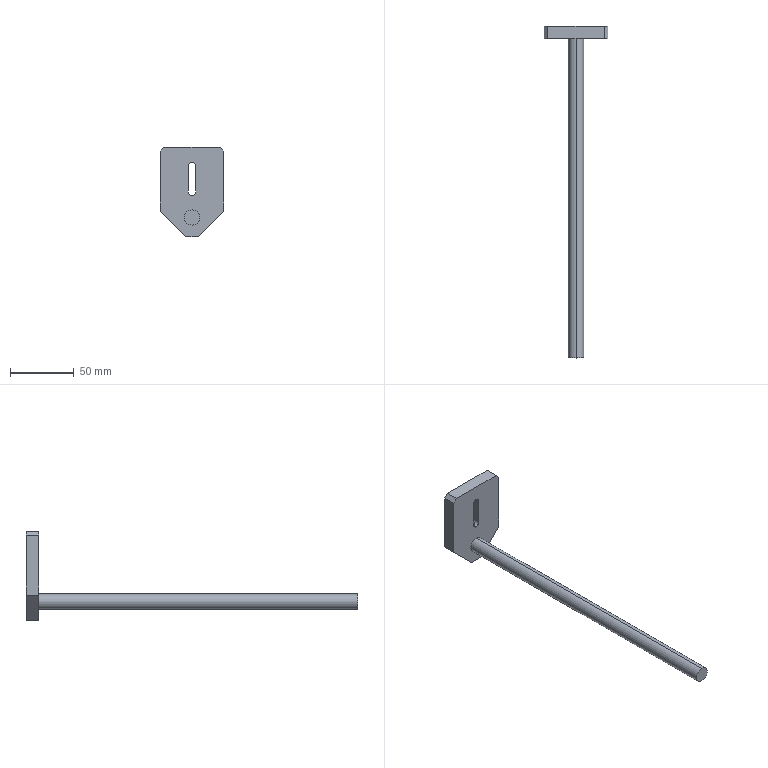Part | SolidWorks | features ICE 3, Chamfer 1, Extrusion 1, HoleWzd 1 | 1 solid | 20 faces | box 50 x 260 x 70 mm | volume 57256 mm3 | plane 13 | cylinder 7 | commonest cylinder face diameters 6 x3 4.2 x2 12 x2
STEP:
#1=CARTESIAN_POINT('',(2.1,5.,-12.142));
#2=VERTEX_POINT('',#1);
#3=CARTESIAN_POINT('',(0.,2.9,-13.));
#4=VERTEX_POINT('',#3);
#5=CARTESIAN_POINT('',(2.1,5.,-12.142));
#6=CARTESIAN_POINT('',(2.1,4.858,-12.142));
#7=CARTESIAN_POINT('',(2.085,4.714,-12.157));
#8=CARTESIAN_POINT('',(2.028,4.438,-12.211));
#9=CARTESIAN_POINT('',(1.986,4.305,-12.249));
#10=CARTESIAN_POINT('',(1.88,4.054,-12.339));
#11=CARTESIAN_POINT('',(1.816,3.937,-12.39));
#12=CARTESIAN_POINT('',(1.668,3.718,-12.495));
#13=CARTESIAN_POINT('',(1.583,3.614,-12.551));
#14=CARTESIAN_POINT('',(1.396,3.426,-12.657));
#15=CARTESIAN_POINT('',(1.295,3.341,-12.709));
#16=CARTESIAN_POINT('',(1.072,3.189,-12.804));
#17=CARTESIAN_POINT('',(0.9508,3.123,-12.848));
#18=CARTESIAN_POINT('',(0.6972,3.014,-12.921));
#19=CARTESIAN_POINT('',(0.5628,2.972,-12.95));
#20=CARTESIAN_POINT('',(0.2837,2.914,-12.99));
#21=CARTESIAN_POINT('',(0.1426,2.9,-13.));
#22=CARTESIAN_POINT('',(0.,2.9,-13.));
#23=B_SPLINE_CURVE_WITH_KNOTS('',3,(#5,#6,#7,#8,#9,#10,#11,#12,#13,#14,#15,#16,#17,#18,#19,#20,#21,#22),.UNSPECIFIED.,.F.,.F.,(4,2,2,2,2,2,2,2,4),(0.006811,0.007236,0.007662,0.008087,0.008512,0.008938,0.009363,0.009789,0.01021),.UNSPECIFIED.);
#24=EDGE_CURVE('',#2,#4,#23,.T.);
#25=ORIENTED_EDGE('',*,*,#24,.F.);
#26=CARTESIAN_POINT('',(2.1,5.,-45.));
#27=VERTEX_POINT('',#26);
#28=CARTESIAN_POINT('',(2.1,5.,-45.));
#29=DIRECTION('',(0.,0.,-1.));
#30=VECTOR('',#29,1000.);
#31=LINE('',#28,#30);
#32=EDGE_CURVE('',#2,#27,#31,.T.);
#33=ORIENTED_EDGE('',*,*,#32,.T.);
#34=CARTESIAN_POINT('',(-2.1,5.,-45.));
#35=VERTEX_POINT('',#34);
#36=CARTESIAN_POINT('',(0.,5.,-45.));
#37=DIRECTION('',(0.,0.,-1.));
#38=DIRECTION('',(-1.,0.,0.));
#39=AXIS2_PLACEMENT_3D('',#36,#37,#38);
#40=CIRCLE('',#39,2.1);
#41=EDGE_CURVE('',#27,#35,#40,.T.);
#42=ORIENTED_EDGE('',*,*,#41,.T.);
#43=CARTESIAN_POINT('',(-2.1,5.,-12.142));
#44=VERTEX_POINT('',#43);
#45=CARTESIAN_POINT('',(-2.1,5.,-45.));
#46=DIRECTION('',(0.,0.,-1.));
#47=VECTOR('',#46,1000.);
#48=LINE('',#45,#47);
#49=EDGE_CURVE('',#44,#35,#48,.T.);
#50=ORIENTED_EDGE('',*,*,#49,.F.);
#51=CARTESIAN_POINT('',(0.,2.9,-13.));
#52=CARTESIAN_POINT('',(-0.1424,2.9,-13.));
#53=CARTESIAN_POINT('',(-0.2871,2.915,-12.989));
#54=CARTESIAN_POINT('',(-0.5634,2.972,-12.95));
#55=CARTESIAN_POINT('',(-0.6985,3.015,-12.921));
#56=CARTESIAN_POINT('',(-1.081,3.178,-12.811));
#57=CARTESIAN_POINT('',(-1.306,3.334,-12.709));
#58=CARTESIAN_POINT('',(-1.678,3.71,-12.496));
#59=CARTESIAN_POINT('',(-1.828,3.933,-12.382));
#60=CARTESIAN_POINT('',(-1.986,4.305,-12.249));
#61=CARTESIAN_POINT('',(-2.028,4.438,-12.211));
#62=CARTESIAN_POINT('',(-2.085,4.714,-12.157));
#63=CARTESIAN_POINT('',(-2.1,4.856,-12.142));
#64=CARTESIAN_POINT('',(-2.1,5.,-12.142));
#65=B_SPLINE_CURVE_WITH_KNOTS('',3,(#51,#52,#53,#54,#55,#56,#57,#58,#59,#60,#61,#62,#63,#64),.UNSPECIFIED.,.F.,.F.,(4,2,2,2,2,2,4),(0.01021,0.01064,0.01106,0.01191,0.01276,0.01319,0.01361),.UNSPECIFIED.);
#66=EDGE_CURVE('',#4,#44,#65,.T.);
#67=ORIENTED_EDGE('',*,*,#66,.F.);
#68=EDGE_LOOP('',(#25,#33,#42,#50,#67));
#69=FACE_OUTER_BOUND('',#68,.T.);
#70=CARTESIAN_POINT('',(0.,5.,-45.));
#71=DIRECTION('',(0.,0.,-1.));
#72=DIRECTION('',(-1.,0.,0.));
#73=AXIS2_PLACEMENT_3D('',#70,#71,#72);
#74=CYLINDRICAL_SURFACE('',#73,2.1);
#75=ADVANCED_FACE('',(#69),#74,.F.);
#76=CARTESIAN_POINT('',(0.,10.,-13.));
#77=VERTEX_POINT('',#76);
#78=CARTESIAN_POINT('',(3.,10.,-10.));
#79=VERTEX_POINT('',#78);
#80=CARTESIAN_POINT('',(0.,10.,-10.));
#81=DIRECTION('',(0.,-1.,0.));
#82=DIRECTION('',(0.,0.,-1.));
#83=AXIS2_PLACEMENT_3D('',#80,#81,#82);
#84=CIRCLE('',#83,3.);
#85=EDGE_CURVE('',#77,#79,#84,.T.);
#86=ORIENTED_EDGE('',*,*,#85,.F.);
#87=CARTESIAN_POINT('',(0.,7.1,-13.));
#88=VERTEX_POINT('',#87);
#89=CARTESIAN_POINT('',(0.,10.,-13.));
#90=DIRECTION('',(0.,-1.,0.));
#91=VECTOR('',#90,1000.);
#92=LINE('',#89,#91);
#93=EDGE_CURVE('',#77,#88,#92,.T.);
#94=ORIENTED_EDGE('',*,*,#93,.T.);
#95=CARTESIAN_POINT('',(0.,7.1,-13.));
#96=CARTESIAN_POINT('',(0.1432,7.1,-13.));
#97=CARTESIAN_POINT('',(0.2844,7.086,-12.99));
#98=CARTESIAN_POINT('',(0.5628,7.028,-12.95));
#99=CARTESIAN_POINT('',(0.6977,6.986,-12.921));
#100=CARTESIAN_POINT('',(0.9516,6.877,-12.848));
#101=CARTESIAN_POINT('',(1.073,6.81,-12.804));
#102=CARTESIAN_POINT('',(1.295,6.658,-12.709));
#103=CARTESIAN_POINT('',(1.397,6.573,-12.657));
#104=CARTESIAN_POINT('',(1.679,6.289,-12.495));
#105=CARTESIAN_POINT('',(1.828,6.07,-12.383));
#106=CARTESIAN_POINT('',(1.987,5.692,-12.249));
#107=CARTESIAN_POINT('',(2.028,5.561,-12.211));
#108=CARTESIAN_POINT('',(2.085,5.285,-12.157));
#109=CARTESIAN_POINT('',(2.1,5.142,-12.142));
#110=CARTESIAN_POINT('',(2.1,5.,-12.142));
#111=B_SPLINE_CURVE_WITH_KNOTS('',3,(#95,#96,#97,#98,#99,#100,#101,#102,#103,#104,#105,#106,#107,#108,#109,#110),.UNSPECIFIED.,.F.,.F.,(4,2,2,2,2,2,2,4),(0.003408,0.003833,0.004259,0.004684,0.005109,0.00596,0.006386,0.006811),.UNSPECIFIED.);
#112=EDGE_CURVE('',#88,#2,#111,.T.);
#113=ORIENTED_EDGE('',*,*,#112,.T.);
#114=ORIENTED_EDGE('',*,*,#24,.T.);
#115=CARTESIAN_POINT('',(0.,0.,-13.));
#116=VERTEX_POINT('',#115);
#117=CARTESIAN_POINT('',(0.,10.,-13.));
#118=DIRECTION('',(0.,-1.,0.));
#119=VECTOR('',#118,1000.);
#120=LINE('',#117,#119);
#121=EDGE_CURVE('',#4,#116,#120,.T.);
#122=ORIENTED_EDGE('',*,*,#121,.T.);
#123=CARTESIAN_POINT('',(3.,0.,-10.));
#124=VERTEX_POINT('',#123);
#125=CARTESIAN_POINT('',(0.,0.,-10.));
#126=DIRECTION('',(0.,-1.,0.));
#127=DIRECTION('',(0.,0.,-1.));
#128=AXIS2_PLACEMENT_3D('',#125,#126,#127);
#129=CIRCLE('',#128,3.);
#130=EDGE_CURVE('',#116,#124,#129,.T.);
#131=ORIENTED_EDGE('',*,*,#130,.T.);
#132=CARTESIAN_POINT('',(3.,10.,-10.));
#133=DIRECTION('',(0.,-1.,0.));
#134=VECTOR('',#133,1000.);
#135=LINE('',#132,#134);
#136=EDGE_CURVE('',#79,#124,#135,.T.);
#137=ORIENTED_EDGE('',*,*,#136,.F.);
#138=EDGE_LOOP('',(#86,#94,#113,#114,#122,#131,#137));
#139=FACE_OUTER_BOUND('',#138,.T.);
#140=CARTESIAN_POINT('',(0.,10.,-10.));
#141=DIRECTION('',(0.,-1.,0.));
#142=DIRECTION('',(0.,0.,-1.));
#143=AXIS2_PLACEMENT_3D('',#140,#141,#142);
#144=CYLINDRICAL_SURFACE('',#143,3.);
#145=ADVANCED_FACE('',(#139),#144,.F.);
#146=CARTESIAN_POINT('',(0.,-250.,-36.));
#147=VERTEX_POINT('',#146);
#148=CARTESIAN_POINT('',(0.,-250.,-24.));
#149=VERTEX_POINT('',#148);
#150=CARTESIAN_POINT('',(0.,-250.,-30.));
#151=DIRECTION('',(0.,-1.,0.));
#152=DIRECTION('',(0.,0.,-1.));
#153=AXIS2_PLACEMENT_3D('',#150,#151,#152);
#154=CIRCLE('',#153,6.);
#155=EDGE_CURVE('',#147,#149,#154,.T.);
#156=ORIENTED_EDGE('',*,*,#155,.F.);
#157=CARTESIAN_POINT('',(0.,0.,-36.));
#158=VERTEX_POINT('',#157);
#159=CARTESIAN_POINT('',(0.,-250.,-36.));
#160=DIRECTION('',(0.,1.,0.));
#161=VECTOR('',#160,1000.);
#162=LINE('',#159,#161);
#163=EDGE_CURVE('',#147,#158,#162,.T.);
#164=ORIENTED_EDGE('',*,*,#163,.T.);
#165=CARTESIAN_POINT('',(0.,0.,-24.));
#166=VERTEX_POINT('',#165);
#167=CARTESIAN_POINT('',(0.,0.,-30.));
#168=DIRECTION('',(0.,-1.,0.));
#169=DIRECTION('',(0.,0.,1.));
#170=AXIS2_PLACEMENT_3D('',#167,#168,#169);
#171=CIRCLE('',#170,6.);
#172=EDGE_CURVE('',#158,#166,#171,.T.);
#173=ORIENTED_EDGE('',*,*,#172,.T.);
#174=CARTESIAN_POINT('',(0.,-250.,-24.));
#175=DIRECTION('',(0.,1.,0.));
#176=VECTOR('',#175,1000.);
#177=LINE('',#174,#176);
#178=EDGE_CURVE('',#149,#166,#177,.T.);
#179=ORIENTED_EDGE('',*,*,#178,.F.);
#180=EDGE_LOOP('',(#156,#164,#173,#179));
#181=FACE_OUTER_BOUND('',#180,.T.);
#182=CARTESIAN_POINT('',(0.,-250.,-30.));
#183=DIRECTION('',(0.,1.,0.));
#184=DIRECTION('',(0.,0.,1.));
#185=AXIS2_PLACEMENT_3D('',#182,#183,#184);
#186=CYLINDRICAL_SURFACE('',#185,6.);
#187=ADVANCED_FACE('',(#181),#186,.T.);
#188=CARTESIAN_POINT('',(25.,0.,-25.));
#189=VERTEX_POINT('',#188);
#190=CARTESIAN_POINT('',(5.,0.,-45.));
#191=VERTEX_POINT('',#190);
#192=CARTESIAN_POINT('',(5.,0.,-45.));
#193=DIRECTION('',(-0.7071,0.,-0.7071));
#194=VECTOR('',#193,1000.);
#195=LINE('',#192,#194);
#196=EDGE_CURVE('',#189,#191,#195,.T.);
#197=ORIENTED_EDGE('',*,*,#196,.T.);
#198=CARTESIAN_POINT('',(5.,10.,-45.));
#199=VERTEX_POINT('',#198);
#200=CARTESIAN_POINT('',(5.,10.,-45.));
#201=DIRECTION('',(0.,-1.,0.));
#202=VECTOR('',#201,1000.);
#203=LINE('',#200,#202);
#204=EDGE_CURVE('',#199,#191,#203,.T.);
#205=ORIENTED_EDGE('',*,*,#204,.F.);
#206=CARTESIAN_POINT('',(25.,10.,-25.));
#207=VERTEX_POINT('',#206);
#208=CARTESIAN_POINT('',(5.,10.,-45.));
#209=DIRECTION('',(-0.7071,0.,-0.7071));
#210=VECTOR('',#209,1000.);
#211=LINE('',#208,#210);
#212=EDGE_CURVE('',#207,#199,#211,.T.);
#213=ORIENTED_EDGE('',*,*,#212,.F.);
#214=CARTESIAN_POINT('',(25.,10.,-25.));
#215=DIRECTION('',(0.,-1.,0.));
#216=VECTOR('',#215,1000.);
#217=LINE('',#214,#216);
#218=EDGE_CURVE('',#207,#189,#217,.T.);
#219=ORIENTED_EDGE('',*,*,#218,.T.);
#220=EDGE_LOOP('',(#197,#205,#213,#219));
#221=FACE_OUTER_BOUND('',#220,.T.);
#222=CARTESIAN_POINT('',(5.,10.,-45.));
#223=DIRECTION('',(-0.7071,0.,0.7071));
#224=DIRECTION('',(0.7071,0.,0.7071));
#225=AXIS2_PLACEMENT_3D('',#222,#223,#224);
#226=PLANE('',#225);
#227=ADVANCED_FACE('',(#221),#226,.F.);
#228=CARTESIAN_POINT('',(0.,5.,-45.));
#229=DIRECTION('',(0.,0.,-1.));
#230=DIRECTION('',(-1.,0.,0.));
#231=AXIS2_PLACEMENT_3D('',#228,#229,#230);
#232=CIRCLE('',#231,2.1);
#233=EDGE_CURVE('',#35,#27,#232,.T.);
#234=ORIENTED_EDGE('',*,*,#233,.F.);
#235=ORIENTED_EDGE('',*,*,#41,.F.);
#236=EDGE_LOOP('',(#234,#235));
#237=FACE_BOUND('',#236,.T.);
#238=CARTESIAN_POINT('',(-5.,0.,-45.));
#239=VERTEX_POINT('',#238);
#240=CARTESIAN_POINT('',(-5.,0.,-45.));
#241=DIRECTION('',(-1.,0.,0.));
#242=VECTOR('',#241,1000.);
#243=LINE('',#240,#242);
#244=EDGE_CURVE('',#191,#239,#243,.T.);
#245=ORIENTED_EDGE('',*,*,#244,.T.);
#246=CARTESIAN_POINT('',(-5.,10.,-45.));
#247=VERTEX_POINT('',#246);
#248=CARTESIAN_POINT('',(-5.,10.,-45.));
#249=DIRECTION('',(0.,-1.,0.));
#250=VECTOR('',#249,1000.);
#251=LINE('',#248,#250);
#252=EDGE_CURVE('',#247,#239,#251,.T.);
#253=ORIENTED_EDGE('',*,*,#252,.F.);
#254=CARTESIAN_POINT('',(-5.,10.,-45.));
#255=DIRECTION('',(-1.,0.,0.));
#256=VECTOR('',#255,1000.);
#257=LINE('',#254,#256);
#258=EDGE_CURVE('',#199,#247,#257,.T.);
#259=ORIENTED_EDGE('',*,*,#258,.F.);
#260=ORIENTED_EDGE('',*,*,#204,.T.);
#261=EDGE_LOOP('',(#245,#253,#259,#260));
#262=FACE_OUTER_BOUND('',#261,.T.);
#263=CARTESIAN_POINT('',(-5.,10.,-45.));
#264=DIRECTION('',(0.,0.,1.));
#265=DIRECTION('',(1.,0.,0.));
#266=AXIS2_PLACEMENT_3D('',#263,#264,#265);
#267=PLANE('',#266);
#268=ADVANCED_FACE('',(#237,#262),#267,.F.);
#269=CARTESIAN_POINT('',(-25.,0.,-25.));
#270=VERTEX_POINT('',#269);
#271=CARTESIAN_POINT('',(-25.,0.,-25.));
#272=DIRECTION('',(-0.7071,0.,0.7071));
#273=VECTOR('',#272,1000.);
#274=LINE('',#271,#273);
#275=EDGE_CURVE('',#239,#270,#274,.T.);
#276=ORIENTED_EDGE('',*,*,#275,.T.);
#277=CARTESIAN_POINT('',(-25.,10.,-25.));
#278=VERTEX_POINT('',#277);
#279=CARTESIAN_POINT('',(-25.,10.,-25.));
#280=DIRECTION('',(0.,-1.,0.));
#281=VECTOR('',#280,1000.);
#282=LINE('',#279,#281);
#283=EDGE_CURVE('',#278,#270,#282,.T.);
#284=ORIENTED_EDGE('',*,*,#283,.F.);
#285=CARTESIAN_POINT('',(-25.,10.,-25.));
#286=DIRECTION('',(-0.7071,0.,0.7071));
#287=VECTOR('',#286,1000.);
#288=LINE('',#285,#287);
#289=EDGE_CURVE('',#247,#278,#288,.T.);
#290=ORIENTED_EDGE('',*,*,#289,.F.);
#291=ORIENTED_EDGE('',*,*,#252,.T.);
#292=EDGE_LOOP('',(#276,#284,#290,#291));
#293=FACE_OUTER_BOUND('',#292,.T.);
#294=CARTESIAN_POINT('',(-25.,10.,-25.));
#295=DIRECTION('',(0.7071,0.,0.7071));
#296=DIRECTION('',(0.7071,0.,-0.7071));
#297=AXIS2_PLACEMENT_3D('',#294,#295,#296);
#298=PLANE('',#297);
#299=ADVANCED_FACE('',(#293),#298,.F.);
#300=CARTESIAN_POINT('',(-25.,0.,22.));
#301=VERTEX_POINT('',#300);
#302=CARTESIAN_POINT('',(-25.,0.,25.));
#303=DIRECTION('',(0.,0.,1.));
#304=VECTOR('',#303,1000.);
#305=LINE('',#302,#304);
#306=EDGE_CURVE('',#270,#301,#305,.T.);
#307=ORIENTED_EDGE('',*,*,#306,.T.);
#308=CARTESIAN_POINT('',(-25.,10.,22.));
#309=VERTEX_POINT('',#308);
#310=CARTESIAN_POINT('',(-25.,10.,22.));
#311=DIRECTION('',(0.,1.,0.));
#312=VECTOR('',#311,1000.);
#313=LINE('',#310,#312);
#314=EDGE_CURVE('',#301,#309,#313,.T.);
#315=ORIENTED_EDGE('',*,*,#314,.T.);
#316=CARTESIAN_POINT('',(-25.,10.,25.));
#317=DIRECTION('',(0.,0.,1.));
#318=VECTOR('',#317,1000.);
#319=LINE('',#316,#318);
#320=EDGE_CURVE('',#278,#309,#319,.T.);
#321=ORIENTED_EDGE('',*,*,#320,.F.);
#322=ORIENTED_EDGE('',*,*,#283,.T.);
#323=EDGE_LOOP('',(#307,#315,#321,#322));
#324=FACE_OUTER_BOUND('',#323,.T.);
#325=CARTESIAN_POINT('',(-25.,10.,25.));
#326=DIRECTION('',(1.,0.,0.));
#327=DIRECTION('',(0.,0.,-1.));
#328=AXIS2_PLACEMENT_3D('',#325,#326,#327);
#329=PLANE('',#328);
#330=ADVANCED_FACE('',(#324),#329,.F.);
#331=CARTESIAN_POINT('',(-22.,10.,25.));
#332=VERTEX_POINT('',#331);
#333=CARTESIAN_POINT('',(22.,10.,25.));
#334=VERTEX_POINT('',#333);
#335=CARTESIAN_POINT('',(-25.,10.,25.));
#336=DIRECTION('',(1.,0.,0.));
#337=VECTOR('',#336,1000.);
#338=LINE('',#335,#337);
#339=EDGE_CURVE('',#332,#334,#338,.T.);
#340=ORIENTED_EDGE('',*,*,#339,.F.);
#341=CARTESIAN_POINT('',(-22.,0.,25.));
#342=VERTEX_POINT('',#341);
#343=CARTESIAN_POINT('',(-22.,10.,25.));
#344=DIRECTION('',(0.,-1.,0.));
#345=VECTOR('',#344,1000.);
#346=LINE('',#343,#345);
#347=EDGE_CURVE('',#332,#342,#346,.T.);
#348=ORIENTED_EDGE('',*,*,#347,.T.);
#349=CARTESIAN_POINT('',(22.,0.,25.));
#350=VERTEX_POINT('',#349);
#351=CARTESIAN_POINT('',(-25.,0.,25.));
#352=DIRECTION('',(1.,0.,0.));
#353=VECTOR('',#352,1000.);
#354=LINE('',#351,#353);
#355=EDGE_CURVE('',#342,#350,#354,.T.);
#356=ORIENTED_EDGE('',*,*,#355,.T.);
#357=CARTESIAN_POINT('',(22.,10.,25.));
#358=DIRECTION('',(0.,1.,0.));
#359=VECTOR('',#358,1000.);
#360=LINE('',#357,#359);
#361=EDGE_CURVE('',#350,#334,#360,.T.);
#362=ORIENTED_EDGE('',*,*,#361,.T.);
#363=EDGE_LOOP('',(#340,#348,#356,#362));
#364=FACE_OUTER_BOUND('',#363,.T.);
#365=CARTESIAN_POINT('',(-25.,10.,25.));
#366=DIRECTION('',(0.,0.,-1.));
#367=DIRECTION('',(-1.,0.,0.));
#368=AXIS2_PLACEMENT_3D('',#365,#366,#367);
#369=PLANE('',#368);
#370=ADVANCED_FACE('',(#364),#369,.F.);
#371=CARTESIAN_POINT('',(25.,10.,22.));
#372=VERTEX_POINT('',#371);
#373=CARTESIAN_POINT('',(25.,10.,25.));
#374=DIRECTION('',(0.,0.,-1.));
#375=VECTOR('',#374,1000.);
#376=LINE('',#373,#375);
#377=EDGE_CURVE('',#372,#207,#376,.T.);
#378=ORIENTED_EDGE('',*,*,#377,.F.);
#379=CARTESIAN_POINT('',(25.,0.,22.));
#380=VERTEX_POINT('',#379);
#381=CARTESIAN_POINT('',(25.,10.,22.));
#382=DIRECTION('',(0.,-1.,0.));
#383=VECTOR('',#382,1000.);
#384=LINE('',#381,#383);
#385=EDGE_CURVE('',#372,#380,#384,.T.);
#386=ORIENTED_EDGE('',*,*,#385,.T.);
#387=CARTESIAN_POINT('',(25.,0.,25.));
#388=DIRECTION('',(0.,0.,-1.));
#389=VECTOR('',#388,1000.);
#390=LINE('',#387,#389);
#391=EDGE_CURVE('',#380,#189,#390,.T.);
#392=ORIENTED_EDGE('',*,*,#391,.T.);
#393=ORIENTED_EDGE('',*,*,#218,.F.);
#394=EDGE_LOOP('',(#378,#386,#392,#393));
#395=FACE_OUTER_BOUND('',#394,.T.);
#396=CARTESIAN_POINT('',(25.,10.,25.));
#397=DIRECTION('',(-1.,0.,0.));
#398=DIRECTION('',(0.,0.,1.));
#399=AXIS2_PLACEMENT_3D('',#396,#397,#398);
#400=PLANE('',#399);
#401=ADVANCED_FACE('',(#395),#400,.F.);
#402=CARTESIAN_POINT('',(-3.,10.,-10.));
#403=VERTEX_POINT('',#402);
#404=CARTESIAN_POINT('',(0.,10.,-10.));
#405=DIRECTION('',(0.,-1.,0.));
#406=DIRECTION('',(0.,0.,-1.));
#407=AXIS2_PLACEMENT_3D('',#404,#405,#406);
#408=CIRCLE('',#407,3.);
#409=EDGE_CURVE('',#403,#77,#408,.T.);
#410=ORIENTED_EDGE('',*,*,#409,.T.);
#411=ORIENTED_EDGE('',*,*,#85,.T.);
#412=CARTESIAN_POINT('',(3.,10.,10.));
#413=VERTEX_POINT('',#412);
#414=CARTESIAN_POINT('',(3.,10.,-10.));
#415=DIRECTION('',(0.,0.,1.));
#416=VECTOR('',#415,1000.);
#417=LINE('',#414,#416);
#418=EDGE_CURVE('',#79,#413,#417,.T.);
#419=ORIENTED_EDGE('',*,*,#418,.T.);
#420=CARTESIAN_POINT('',(-3.,10.,10.));
#421=VERTEX_POINT('',#420);
#422=CARTESIAN_POINT('',(0.,10.,10.));
#423=DIRECTION('',(0.,-1.,0.));
#424=DIRECTION('',(0.,0.,-1.));
#425=AXIS2_PLACEMENT_3D('',#422,#423,#424);
#426=CIRCLE('',#425,3.);
#427=EDGE_CURVE('',#413,#421,#426,.T.);
#428=ORIENTED_EDGE('',*,*,#427,.T.);
#429=CARTESIAN_POINT('',(-3.,10.,-10.));
#430=DIRECTION('',(0.,0.,-1.));
#431=VECTOR('',#430,1000.);
#432=LINE('',#429,#431);
#433=EDGE_CURVE('',#421,#403,#432,.T.);
#434=ORIENTED_EDGE('',*,*,#433,.T.);
#435=EDGE_LOOP('',(#410,#411,#419,#428,#434));
#436=FACE_BOUND('',#435,.T.);
#437=ORIENTED_EDGE('',*,*,#320,.T.);
#438=CARTESIAN_POINT('',(-23.5,10.,23.5));
#439=DIRECTION('',(0.7071,0.,0.7071));
#440=VECTOR('',#439,1000.);
#441=LINE('',#438,#440);
#442=EDGE_CURVE('',#309,#332,#441,.T.);
#443=ORIENTED_EDGE('',*,*,#442,.T.);
#444=ORIENTED_EDGE('',*,*,#339,.T.);
#445=CARTESIAN_POINT('',(23.5,10.,23.5));
#446=DIRECTION('',(0.7071,0.,-0.7071));
#447=VECTOR('',#446,1000.);
#448=LINE('',#445,#447);
#449=EDGE_CURVE('',#334,#372,#448,.T.);
#450=ORIENTED_EDGE('',*,*,#449,.T.);
#451=ORIENTED_EDGE('',*,*,#377,.T.);
#452=ORIENTED_EDGE('',*,*,#212,.T.);
#453=ORIENTED_EDGE('',*,*,#258,.T.);
#454=ORIENTED_EDGE('',*,*,#289,.T.);
#455=EDGE_LOOP('',(#437,#443,#444,#450,#451,#452,#453,#454));
#456=FACE_OUTER_BOUND('',#455,.T.);
#457=CARTESIAN_POINT('',(0.,10.,0.));
#458=DIRECTION('',(0.,1.,0.));
#459=DIRECTION('',(0.,0.,1.));
#460=AXIS2_PLACEMENT_3D('',#457,#458,#459);
#461=PLANE('',#460);
#462=ADVANCED_FACE('',(#436,#456),#461,.T.);
#463=CARTESIAN_POINT('',(3.,0.,10.));
#464=VERTEX_POINT('',#463);
#465=CARTESIAN_POINT('',(3.,0.,-10.));
#466=DIRECTION('',(0.,0.,1.));
#467=VECTOR('',#466,1000.);
#468=LINE('',#465,#467);
#469=EDGE_CURVE('',#124,#464,#468,.T.);
#470=ORIENTED_EDGE('',*,*,#469,.F.);
#471=ORIENTED_EDGE('',*,*,#130,.F.);
#472=CARTESIAN_POINT('',(-3.,0.,-10.));
#473=VERTEX_POINT('',#472);
#474=CARTESIAN_POINT('',(0.,0.,-10.));
#475=DIRECTION('',(0.,-1.,0.));
#476=DIRECTION('',(0.,0.,-1.));
#477=AXIS2_PLACEMENT_3D('',#474,#475,#476);
#478=CIRCLE('',#477,3.);
#479=EDGE_CURVE('',#473,#116,#478,.T.);
#480=ORIENTED_EDGE('',*,*,#479,.F.);
#481=CARTESIAN_POINT('',(-3.,0.,10.));
#482=VERTEX_POINT('',#481);
#483=CARTESIAN_POINT('',(-3.,0.,-10.));
#484=DIRECTION('',(0.,0.,-1.));
#485=VECTOR('',#484,1000.);
#486=LINE('',#483,#485);
#487=EDGE_CURVE('',#482,#473,#486,.T.);
#488=ORIENTED_EDGE('',*,*,#487,.F.);
#489=CARTESIAN_POINT('',(0.,0.,10.));
#490=DIRECTION('',(0.,-1.,0.));
#491=DIRECTION('',(0.,0.,-1.));
#492=AXIS2_PLACEMENT_3D('',#489,#490,#491);
#493=CIRCLE('',#492,3.);
#494=EDGE_CURVE('',#464,#482,#493,.T.);
#495=ORIENTED_EDGE('',*,*,#494,.F.);
#496=EDGE_LOOP('',(#470,#471,#480,#488,#495));
#497=FACE_BOUND('',#496,.T.);
#498=CARTESIAN_POINT('',(0.,0.,-30.));
#499=DIRECTION('',(0.,-1.,0.));
#500=DIRECTION('',(0.,0.,1.));
#501=AXIS2_PLACEMENT_3D('',#498,#499,#500);
#502=CIRCLE('',#501,6.);
#503=EDGE_CURVE('',#166,#158,#502,.T.);
#504=ORIENTED_EDGE('',*,*,#503,.F.);
#505=ORIENTED_EDGE('',*,*,#172,.F.);
#506=EDGE_LOOP('',(#504,#505));
#507=FACE_BOUND('',#506,.T.);
#508=ORIENTED_EDGE('',*,*,#355,.F.);
#509=CARTESIAN_POINT('',(-22.,0.,25.));
#510=DIRECTION('',(-0.7071,0.,-0.7071));
#511=VECTOR('',#510,1000.);
#512=LINE('',#509,#511);
#513=EDGE_CURVE('',#342,#301,#512,.T.);
#514=ORIENTED_EDGE('',*,*,#513,.T.);
#515=ORIENTED_EDGE('',*,*,#306,.F.);
#516=ORIENTED_EDGE('',*,*,#275,.F.);
#517=ORIENTED_EDGE('',*,*,#244,.F.);
#518=ORIENTED_EDGE('',*,*,#196,.F.);
#519=ORIENTED_EDGE('',*,*,#391,.F.);
#520=CARTESIAN_POINT('',(25.,0.,22.));
#521=DIRECTION('',(-0.7071,0.,0.7071));
#522=VECTOR('',#521,1000.);
#523=LINE('',#520,#522);
#524=EDGE_CURVE('',#380,#350,#523,.T.);
#525=ORIENTED_EDGE('',*,*,#524,.T.);
#526=EDGE_LOOP('',(#508,#514,#515,#516,#517,#518,#519,#525));
#527=FACE_OUTER_BOUND('',#526,.T.);
#528=CARTESIAN_POINT('',(0.,0.,0.));
#529=DIRECTION('',(0.,1.,0.));
#530=DIRECTION('',(0.,0.,1.));
#531=AXIS2_PLACEMENT_3D('',#528,#529,#530);
#532=PLANE('',#531);
#533=ADVANCED_FACE('',(#497,#507,#527),#532,.F.);
#534=ORIENTED_EDGE('',*,*,#163,.F.);
#535=CARTESIAN_POINT('',(0.,-250.,-30.));
#536=DIRECTION('',(0.,-1.,0.));
#537=DIRECTION('',(0.,0.,-1.));
#538=AXIS2_PLACEMENT_3D('',#535,#536,#537);
#539=CIRCLE('',#538,6.);
#540=EDGE_CURVE('',#149,#147,#539,.T.);
#541=ORIENTED_EDGE('',*,*,#540,.F.);
#542=ORIENTED_EDGE('',*,*,#178,.T.);
#543=ORIENTED_EDGE('',*,*,#503,.T.);
#544=EDGE_LOOP('',(#534,#541,#542,#543));
#545=FACE_OUTER_BOUND('',#544,.T.);
#546=CARTESIAN_POINT('',(0.,-250.,-30.));
#547=DIRECTION('',(0.,1.,0.));
#548=DIRECTION('',(0.,0.,1.));
#549=AXIS2_PLACEMENT_3D('',#546,#547,#548);
#550=CYLINDRICAL_SURFACE('',#549,6.);
#551=ADVANCED_FACE('',(#545),#550,.T.);
#552=ORIENTED_EDGE('',*,*,#540,.T.);
#553=ORIENTED_EDGE('',*,*,#155,.T.);
#554=EDGE_LOOP('',(#552,#553));
#555=FACE_OUTER_BOUND('',#554,.T.);
#556=CARTESIAN_POINT('',(0.,-250.,-30.));
#557=DIRECTION('',(0.,-1.,0.));
#558=DIRECTION('',(0.,0.,-1.));
#559=AXIS2_PLACEMENT_3D('',#556,#557,#558);
#560=PLANE('',#559);
#561=ADVANCED_FACE('',(#555),#560,.T.);
#562=ORIENTED_EDGE('',*,*,#93,.F.);
#563=ORIENTED_EDGE('',*,*,#409,.F.);
#564=CARTESIAN_POINT('',(-3.,10.,-10.));
#565=DIRECTION('',(0.,-1.,0.));
#566=VECTOR('',#565,1000.);
#567=LINE('',#564,#566);
#568=EDGE_CURVE('',#403,#473,#567,.T.);
#569=ORIENTED_EDGE('',*,*,#568,.T.);
#570=ORIENTED_EDGE('',*,*,#479,.T.);
#571=ORIENTED_EDGE('',*,*,#121,.F.);
#572=ORIENTED_EDGE('',*,*,#66,.T.);
#573=CARTESIAN_POINT('',(-2.1,5.,-12.142));
#574=CARTESIAN_POINT('',(-2.1,5.145,-12.142));
#575=CARTESIAN_POINT('',(-2.085,5.285,-12.157));
#576=CARTESIAN_POINT('',(-2.029,5.56,-12.21));
#577=CARTESIAN_POINT('',(-1.987,5.694,-12.249));
#578=CARTESIAN_POINT('',(-1.828,6.068,-12.383));
#579=CARTESIAN_POINT('',(-1.677,6.291,-12.497));
#580=CARTESIAN_POINT('',(-1.397,6.573,-12.657));
#581=CARTESIAN_POINT('',(-1.293,6.66,-12.71));
#582=CARTESIAN_POINT('',(-1.072,6.811,-12.805));
#583=CARTESIAN_POINT('',(-0.9538,6.876,-12.847));
#584=CARTESIAN_POINT('',(-0.7002,6.985,-12.92));
#585=CARTESIAN_POINT('',(-0.5641,7.028,-12.95));
#586=CARTESIAN_POINT('',(-0.2875,7.085,-12.989));
#587=CARTESIAN_POINT('',(-0.1435,7.1,-13.));
#588=CARTESIAN_POINT('',(0.,7.1,-13.));
#589=B_SPLINE_CURVE_WITH_KNOTS('',3,(#573,#574,#575,#576,#577,#578,#579,#580,#581,#582,#583,#584,#585,#586,#587,#588),.UNSPECIFIED.,.F.,.F.,(4,2,2,2,2,2,2,4),(0.,0.000426,0.000852,0.001704,0.00213,0.002556,0.002982,0.003408),.UNSPECIFIED.);
#590=EDGE_CURVE('',#44,#88,#589,.T.);
#591=ORIENTED_EDGE('',*,*,#590,.T.);
#592=EDGE_LOOP('',(#562,#563,#569,#570,#571,#572,#591));
#593=FACE_OUTER_BOUND('',#592,.T.);
#594=CARTESIAN_POINT('',(0.,10.,-10.));
#595=DIRECTION('',(0.,-1.,0.));
#596=DIRECTION('',(0.,0.,-1.));
#597=AXIS2_PLACEMENT_3D('',#594,#595,#596);
#598=CYLINDRICAL_SURFACE('',#597,3.);
#599=ADVANCED_FACE('',(#593),#598,.F.);
#600=ORIENTED_EDGE('',*,*,#487,.T.);
#601=ORIENTED_EDGE('',*,*,#568,.F.);
#602=ORIENTED_EDGE('',*,*,#433,.F.);
#603=CARTESIAN_POINT('',(-3.,10.,10.));
#604=DIRECTION('',(0.,-1.,0.));
#605=VECTOR('',#604,1000.);
#606=LINE('',#603,#605);
#607=EDGE_CURVE('',#421,#482,#606,.T.);
#608=ORIENTED_EDGE('',*,*,#607,.T.);
#609=EDGE_LOOP('',(#600,#601,#602,#608));
#610=FACE_OUTER_BOUND('',#609,.T.);
#611=CARTESIAN_POINT('',(-3.,10.,-10.));
#612=DIRECTION('',(-1.,0.,0.));
#613=DIRECTION('',(0.,0.,1.));
#614=AXIS2_PLACEMENT_3D('',#611,#612,#613);
#615=PLANE('',#614);
#616=ADVANCED_FACE('',(#610),#615,.F.);
#617=ORIENTED_EDGE('',*,*,#494,.T.);
#618=ORIENTED_EDGE('',*,*,#607,.F.);
#619=ORIENTED_EDGE('',*,*,#427,.F.);
#620=CARTESIAN_POINT('',(3.,10.,10.));
#621=DIRECTION('',(0.,-1.,0.));
#622=VECTOR('',#621,1000.);
#623=LINE('',#620,#622);
#624=EDGE_CURVE('',#413,#464,#623,.T.);
#625=ORIENTED_EDGE('',*,*,#624,.T.);
#626=EDGE_LOOP('',(#617,#618,#619,#625));
#627=FACE_OUTER_BOUND('',#626,.T.);
#628=CARTESIAN_POINT('',(0.,10.,10.));
#629=DIRECTION('',(0.,-1.,0.));
#630=DIRECTION('',(0.,0.,-1.));
#631=AXIS2_PLACEMENT_3D('',#628,#629,#630);
#632=CYLINDRICAL_SURFACE('',#631,3.);
#633=ADVANCED_FACE('',(#627),#632,.F.);
#634=ORIENTED_EDGE('',*,*,#469,.T.);
#635=ORIENTED_EDGE('',*,*,#624,.F.);
#636=ORIENTED_EDGE('',*,*,#418,.F.);
#637=ORIENTED_EDGE('',*,*,#136,.T.);
#638=EDGE_LOOP('',(#634,#635,#636,#637));
#639=FACE_OUTER_BOUND('',#638,.T.);
#640=CARTESIAN_POINT('',(3.,10.,-10.));
#641=DIRECTION('',(1.,0.,0.));
#642=DIRECTION('',(0.,0.,-1.));
#643=AXIS2_PLACEMENT_3D('',#640,#641,#642);
#644=PLANE('',#643);
#645=ADVANCED_FACE('',(#639),#644,.F.);
#646=ORIENTED_EDGE('',*,*,#32,.F.);
#647=ORIENTED_EDGE('',*,*,#112,.F.);
#648=ORIENTED_EDGE('',*,*,#590,.F.);
#649=ORIENTED_EDGE('',*,*,#49,.T.);
#650=ORIENTED_EDGE('',*,*,#233,.T.);
#651=EDGE_LOOP('',(#646,#647,#648,#649,#650));
#652=FACE_OUTER_BOUND('',#651,.T.);
#653=CARTESIAN_POINT('',(0.,5.,-45.));
#654=DIRECTION('',(0.,0.,-1.));
#655=DIRECTION('',(-1.,0.,0.));
#656=AXIS2_PLACEMENT_3D('',#653,#654,#655);
#657=CYLINDRICAL_SURFACE('',#656,2.1);
#658=ADVANCED_FACE('',(#652),#657,.F.);
#659=ORIENTED_EDGE('',*,*,#442,.F.);
#660=ORIENTED_EDGE('',*,*,#314,.F.);
#661=ORIENTED_EDGE('',*,*,#513,.F.);
#662=ORIENTED_EDGE('',*,*,#347,.F.);
#663=EDGE_LOOP('',(#659,#660,#661,#662));
#664=FACE_OUTER_BOUND('',#663,.T.);
#665=CARTESIAN_POINT('',(-22.,10.,25.));
#666=DIRECTION('',(0.7071,0.,-0.7071));
#667=DIRECTION('',(0.,-1.,0.));
#668=AXIS2_PLACEMENT_3D('',#665,#666,#667);
#669=PLANE('',#668);
#670=ADVANCED_FACE('',(#664),#669,.F.);
#671=ORIENTED_EDGE('',*,*,#449,.F.);
#672=ORIENTED_EDGE('',*,*,#361,.F.);
#673=ORIENTED_EDGE('',*,*,#524,.F.);
#674=ORIENTED_EDGE('',*,*,#385,.F.);
#675=EDGE_LOOP('',(#671,#672,#673,#674));
#676=FACE_OUTER_BOUND('',#675,.T.);
#677=CARTESIAN_POINT('',(25.,10.,22.));
#678=DIRECTION('',(-0.7071,0.,-0.7071));
#679=DIRECTION('',(0.,-1.,0.));
#680=AXIS2_PLACEMENT_3D('',#677,#678,#679);
#681=PLANE('',#680);
#682=ADVANCED_FACE('',(#676),#681,.F.);
#683=CLOSED_SHELL('',(#75,#145,#187,#227,#268,#299,#330,#370,#401,#462,#533,#551,#561,#599,#616,#633,#645,#658,#670,#682));
#684=MANIFOLD_SOLID_BREP('',#683);
#685=CARTESIAN_POINT('',(0.,0.,0.));
#686=DIRECTION('',(0.,0.,1.));
#687=DIRECTION('',(1.,0.,0.));
#688=AXIS2_PLACEMENT_3D('',#685,#686,#687);
#689=(LENGTH_UNIT()NAMED_UNIT(*)SI_UNIT(.MILLI.,.METRE.));
#690=UNCERTAINTY_MEASURE_WITH_UNIT(LENGTH_MEASURE(0.00001),#689,'','');
#691=(NAMED_UNIT(*)PLANE_ANGLE_UNIT()SI_UNIT($,.RADIAN.));
#692=(NAMED_UNIT(*)SI_UNIT($,.STERADIAN.)SOLID_ANGLE_UNIT());
#693=(GEOMETRIC_REPRESENTATION_CONTEXT(3)GLOBAL_UNCERTAINTY_ASSIGNED_CONTEXT((#690))GLOBAL_UNIT_ASSIGNED_CONTEXT((#689,#691,#692))REPRESENTATION_CONTEXT('',''));
#694=ADVANCED_BREP_SHAPE_REPRESENTATION('',(#684,#688),#693);